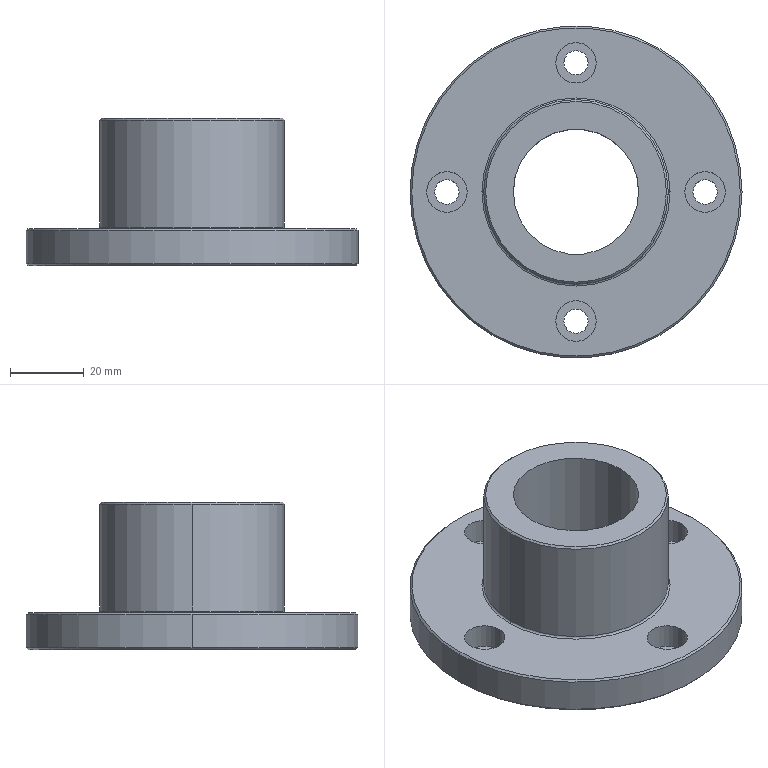Part | STEP file | 44-02-20 Press Cylinder Connector | 1 solid | 37 faces | box 90 x 90 x 40 mm | volume 83101 mm3 | cylinder 22 | plane 7 | cone 6 | torus 2 | commonest cylinder face diameters 6.6 x8 11 x8 34 x2 50 x2 90 x2